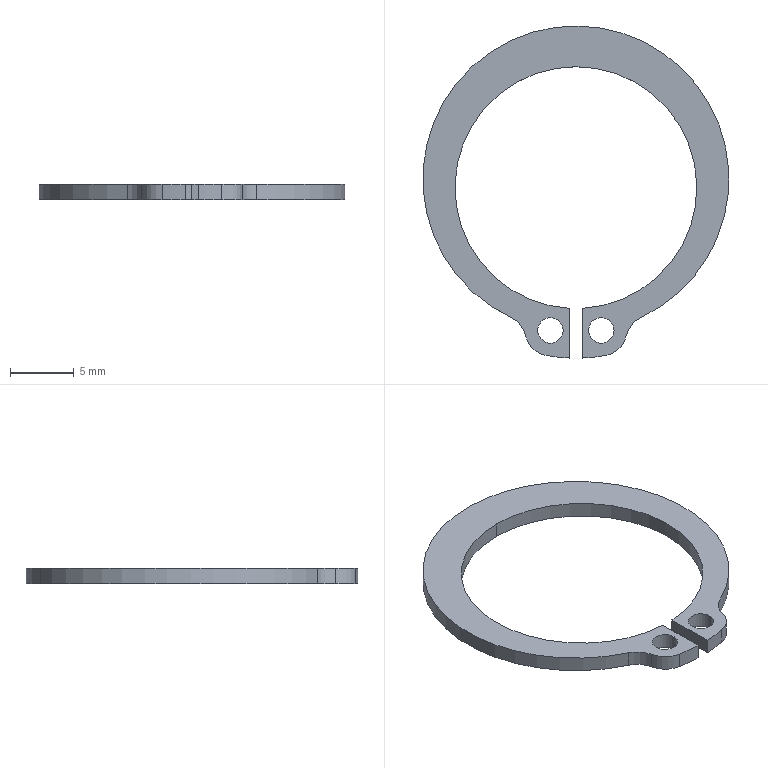Part | STEP file | KS B 1336 - 20 x 1.2 | 1 solid | 18 faces | box 24.05 x 26.087 x 1.2 mm | volume 211.892 mm3 | cylinder 14 | plane 4 | commonest cylinder face diameters 2 x4 4 x4 19 x2 24.05 x2 26.792 x2